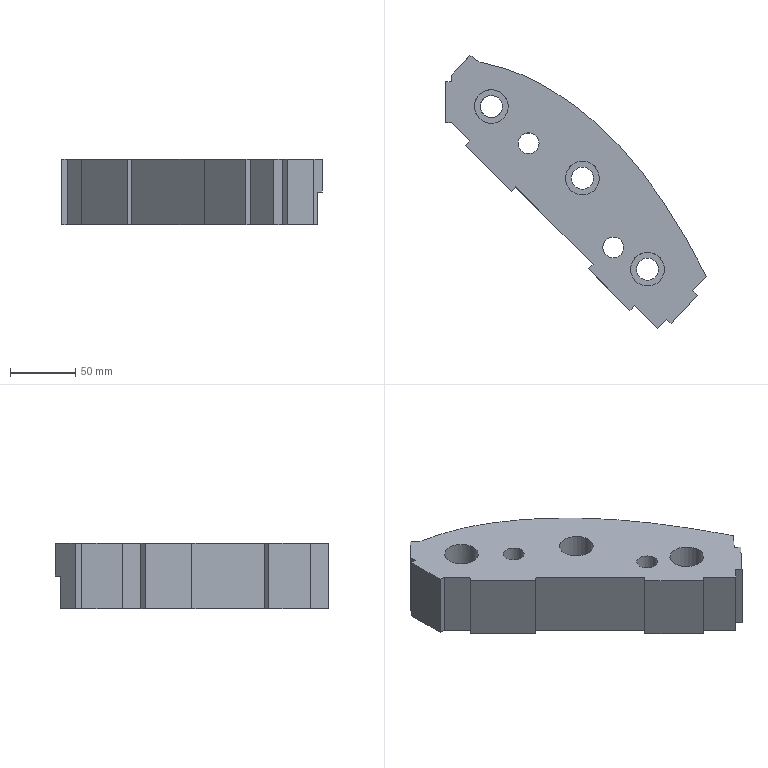Part | NX | features solid 2 | 1 solid | 37 faces | box 200.345 x 210.054 x 50 mm | volume 771106 mm3 | plane 25 | cylinder 8 | spline 4 | commonest cylinder face diameters 17 x3 26 x3 16 x2
STEP:
#1=CARTESIAN_POINT('',(339.431,588.896,-50.));
#2=VERTEX_POINT('',#1);
#3=CARTESIAN_POINT('',(339.431,583.896,-50.));
#4=VERTEX_POINT('',#3);
#5=CARTESIAN_POINT('',(339.431,588.896,-50.));
#6=DIRECTION('',(0.,-1.,0.));
#7=VECTOR('',#6,1000.);
#8=LINE('',#5,#7);
#9=EDGE_CURVE('',#2,#4,#8,.T.);
#10=ORIENTED_EDGE('',*,*,#9,.T.);
#11=CARTESIAN_POINT('',(339.431,583.896,0.));
#12=VERTEX_POINT('',#11);
#13=CARTESIAN_POINT('',(339.431,583.896,-50.));
#14=DIRECTION('',(0.,0.,1.));
#15=VECTOR('',#14,1000.);
#16=LINE('',#13,#15);
#17=EDGE_CURVE('',#4,#12,#16,.T.);
#18=ORIENTED_EDGE('',*,*,#17,.T.);
#19=CARTESIAN_POINT('',(339.431,588.896,0.));
#20=VERTEX_POINT('',#19);
#21=CARTESIAN_POINT('',(339.431,588.896,0.));
#22=DIRECTION('',(0.,-1.,0.));
#23=VECTOR('',#22,1000.);
#24=LINE('',#21,#23);
#25=EDGE_CURVE('',#20,#12,#24,.T.);
#26=ORIENTED_EDGE('',*,*,#25,.F.);
#27=CARTESIAN_POINT('',(339.431,588.896,-50.));
#28=DIRECTION('',(0.,0.,1.));
#29=VECTOR('',#28,1000.);
#30=LINE('',#27,#29);
#31=EDGE_CURVE('',#2,#20,#30,.T.);
#32=ORIENTED_EDGE('',*,*,#31,.F.);
#33=EDGE_LOOP('',(#10,#18,#26,#32));
#34=FACE_BOUND('',#33,.T.);
#35=CARTESIAN_POINT('',(339.431,588.896,-50.));
#36=DIRECTION('',(-1.,0.,0.));
#37=DIRECTION('',(0.,-1.,0.));
#38=AXIS2_PLACEMENT_3D('',#35,#36,#37);
#39=PLANE('',#38);
#40=ADVANCED_FACE('',(#34),#39,.T.);
#41=CARTESIAN_POINT('',(524.901,423.149,0.));
#42=VERTEX_POINT('',#41);
#43=CARTESIAN_POINT('',(535.345,434.348,0.));
#44=VERTEX_POINT('',#43);
#45=CARTESIAN_POINT('',(497.822,394.11,0.));
#46=DIRECTION('',(0.682,0.7314,0.));
#47=VECTOR('',#46,1000.);
#48=LINE('',#45,#47);
#49=EDGE_CURVE('',#42,#44,#48,.T.);
#50=ORIENTED_EDGE('',*,*,#49,.F.);
#51=CARTESIAN_POINT('',(524.901,423.149,-50.));
#52=VERTEX_POINT('',#51);
#53=CARTESIAN_POINT('',(524.901,423.149,-42.5));
#54=DIRECTION('',(0.,0.,1.));
#55=VECTOR('',#54,1000.);
#56=LINE('',#53,#55);
#57=EDGE_CURVE('',#52,#42,#56,.T.);
#58=ORIENTED_EDGE('',*,*,#57,.F.);
#59=CARTESIAN_POINT('',(531.721,430.462,-50.));
#60=VERTEX_POINT('',#59);
#61=CARTESIAN_POINT('',(497.822,394.11,-50.));
#62=DIRECTION('',(0.682,0.7314,0.));
#63=VECTOR('',#62,1000.);
#64=LINE('',#61,#63);
#65=EDGE_CURVE('',#52,#60,#64,.T.);
#66=ORIENTED_EDGE('',*,*,#65,.T.);
#67=CARTESIAN_POINT('',(531.721,430.462,-25.));
#68=VERTEX_POINT('',#67);
#69=CARTESIAN_POINT('',(531.721,430.462,-42.5));
#70=DIRECTION('',(0.,0.,-1.));
#71=VECTOR('',#70,1000.);
#72=LINE('',#69,#71);
#73=EDGE_CURVE('',#60,#68,#72,.F.);
#74=ORIENTED_EDGE('',*,*,#73,.T.);
#75=CARTESIAN_POINT('',(535.345,434.348,-25.));
#76=VERTEX_POINT('',#75);
#77=CARTESIAN_POINT('',(497.822,394.11,-25.));
#78=DIRECTION('',(-0.682,-0.7314,0.));
#79=VECTOR('',#78,1000.);
#80=LINE('',#77,#79);
#81=EDGE_CURVE('',#76,#68,#80,.T.);
#82=ORIENTED_EDGE('',*,*,#81,.F.);
#83=CARTESIAN_POINT('',(535.345,434.348,-50.));
#84=DIRECTION('',(0.,0.,1.));
#85=VECTOR('',#84,1000.);
#86=LINE('',#83,#85);
#87=EDGE_CURVE('',#76,#44,#86,.T.);
#88=ORIENTED_EDGE('',*,*,#87,.T.);
#89=EDGE_LOOP('',(#50,#58,#66,#74,#82,#88));
#90=FACE_BOUND('',#89,.T.);
#91=CARTESIAN_POINT('',(497.822,394.11,-50.));
#92=DIRECTION('',(0.7314,-0.682,0.));
#93=DIRECTION('',(0.682,0.7314,0.));
#94=AXIS2_PLACEMENT_3D('',#91,#92,#93);
#95=PLANE('',#94);
#96=ADVANCED_FACE('',(#90),#95,.T.);
#97=CARTESIAN_POINT('',(471.782,456.506,-50.));
#98=VERTEX_POINT('',#97);
#99=CARTESIAN_POINT('',(463.782,456.506,-50.));
#100=DIRECTION('',(0.,0.,1.));
#101=DIRECTION('',(1.,0.,0.));
#102=AXIS2_PLACEMENT_3D('',#99,#100,#101);
#103=CIRCLE('',#102,8.);
#104=EDGE_CURVE('',#98,#98,#103,.T.);
#105=ORIENTED_EDGE('',*,*,#104,.T.);
#106=EDGE_LOOP('',(#105));
#107=FACE_BOUND('',#106,.T.);
#108=CARTESIAN_POINT('',(406.782,536.506,-50.));
#109=VERTEX_POINT('',#108);
#110=CARTESIAN_POINT('',(398.782,536.506,-50.));
#111=DIRECTION('',(0.,0.,1.));
#112=DIRECTION('',(1.,0.,0.));
#113=AXIS2_PLACEMENT_3D('',#110,#111,#112);
#114=CIRCLE('',#113,8.);
#115=EDGE_CURVE('',#109,#109,#114,.T.);
#116=ORIENTED_EDGE('',*,*,#115,.T.);
#117=EDGE_LOOP('',(#116));
#118=FACE_BOUND('',#117,.T.);
#119=CARTESIAN_POINT('',(498.622,439.794,-50.));
#120=VERTEX_POINT('',#119);
#121=CARTESIAN_POINT('',(490.122,439.794,-50.));
#122=DIRECTION('',(0.,0.,1.));
#123=DIRECTION('',(1.,0.,0.));
#124=AXIS2_PLACEMENT_3D('',#121,#122,#123);
#125=CIRCLE('',#124,8.5);
#126=EDGE_CURVE('',#120,#120,#125,.T.);
#127=ORIENTED_EDGE('',*,*,#126,.T.);
#128=EDGE_LOOP('',(#127));
#129=FACE_BOUND('',#128,.T.);
#130=CARTESIAN_POINT('',(414.032,572.939,-50.));
#131=VERTEX_POINT('',#130);
#132=CARTESIAN_POINT('',(414.032,572.939,-50.));
#133=CARTESIAN_POINT('',(417.217,571.026,-50.));
#134=CARTESIAN_POINT('',(423.539,566.983,-50.));
#135=CARTESIAN_POINT('',(432.884,560.264,-50.));
#136=CARTESIAN_POINT('',(440.545,554.13,-50.));
#137=CARTESIAN_POINT('',(445.865,549.533,-50.));
#138=CARTESIAN_POINT('',(448.857,546.853,-50.));
#139=CARTESIAN_POINT('',(451.177,544.723,-50.));
#140=CARTESIAN_POINT('',(453.165,542.856,-50.));
#141=CARTESIAN_POINT('',(455.911,540.224,-50.));
#142=CARTESIAN_POINT('',(460.621,535.563,-50.));
#143=CARTESIAN_POINT('',(467.258,528.576,-50.));
#144=CARTESIAN_POINT('',(473.713,521.213,-50.));
#145=CARTESIAN_POINT('',(478.166,515.824,-50.));
#146=CARTESIAN_POINT('',(480.658,512.722,-50.));
#147=CARTESIAN_POINT('',(482.595,510.261,-50.));
#148=CARTESIAN_POINT('',(484.212,508.169,-50.));
#149=CARTESIAN_POINT('',(486.473,505.196,-50.));
#150=CARTESIAN_POINT('',(490.365,499.944,-50.));
#151=CARTESIAN_POINT('',(494.805,493.652,-50.));
#152=CARTESIAN_POINT('',(499.205,487.109,-50.));
#153=CARTESIAN_POINT('',(502.491,482.067,-50.));
#154=CARTESIAN_POINT('',(505.213,477.765,-50.));
#155=CARTESIAN_POINT('',(507.12,474.681,-50.));
#156=CARTESIAN_POINT('',(508.194,472.926,-50.));
#157=CARTESIAN_POINT('',(509.037,471.536,-50.));
#158=CARTESIAN_POINT('',(509.729,470.388,-50.));
#159=CARTESIAN_POINT('',(510.707,468.757,-50.));
#160=CARTESIAN_POINT('',(512.396,465.911,-50.));
#161=CARTESIAN_POINT('',(514.835,461.725,-50.));
#162=CARTESIAN_POINT('',(517.278,457.431,-50.));
#163=CARTESIAN_POINT('',(519.009,454.334,-50.));
#164=CARTESIAN_POINT('',(519.981,452.582,-50.));
#165=CARTESIAN_POINT('',(520.767,451.155,-50.));
#166=CARTESIAN_POINT('',(521.338,450.114,-50.));
#167=CARTESIAN_POINT('',(522.19,448.552,-50.));
#168=CARTESIAN_POINT('',(523.25,446.593,-50.));
#169=CARTESIAN_POINT('',(524.572,444.13,-50.));
#170=CARTESIAN_POINT('',(526.378,440.732,-50.));
#171=CARTESIAN_POINT('',(528.729,436.256,-50.));
#172=CARTESIAN_POINT('',(530.708,432.434,-50.));
#173=CARTESIAN_POINT('',(531.721,430.462,-50.));
#174=B_SPLINE_CURVE_WITH_KNOTS('',3,(#132,#133,#134,#135,#136,#137,#138,#139,#140,#141,#142,#143,#144,#145,#146,#147,#148,#149,#150,#151,#152,#153,#154,#155,#156,#157,#158,#159,#160,#161,#162,#163,#164,#165,#166,#167,#168,#169,#170,#171,#172,#173),.UNSPECIFIED.,.F.,.F.,(4,1,1,1,1,1,1,1,1,1,1,1,1,1,1,1,1,1,1,1,1,1,1,1,1,1,1,1,1,1,1,1,1,1,1,1,1,1,1,4),(0.,0.0625,0.125,0.1875,0.2188,0.2344,0.25,0.2656,0.2812,0.3125,0.375,0.4375,0.4688,0.4844,0.5,0.5156,0.5312,0.5625,0.625,0.6562,0.6875,0.7188,0.7344,0.7422,0.75,0.7578,0.7656,0.7812,0.8125,0.8438,0.8594,0.8672,0.875,0.8828,0.8906,0.9062,0.9219,0.9375,0.9688,1.),.UNSPECIFIED.);
#175=EDGE_CURVE('',#60,#131,#174,.F.);
#176=ORIENTED_EDGE('',*,*,#175,.F.);
#177=ORIENTED_EDGE('',*,*,#65,.F.);
#178=CARTESIAN_POINT('',(528.558,419.739,-50.));
#179=VERTEX_POINT('',#178);
#180=CARTESIAN_POINT('',(528.558,419.739,-50.));
#181=DIRECTION('',(-0.7314,0.682,0.));
#182=VECTOR('',#181,1000.);
#183=LINE('',#180,#182);
#184=EDGE_CURVE('',#179,#52,#183,.T.);
#185=ORIENTED_EDGE('',*,*,#184,.F.);
#186=CARTESIAN_POINT('',(508.299,398.013,-50.));
#187=VERTEX_POINT('',#186);
#188=CARTESIAN_POINT('',(501.479,390.7,-50.));
#189=DIRECTION('',(0.682,0.7314,0.));
#190=VECTOR('',#189,1000.);
#191=LINE('',#188,#190);
#192=EDGE_CURVE('',#187,#179,#191,.T.);
#193=ORIENTED_EDGE('',*,*,#192,.F.);
#194=CARTESIAN_POINT('',(504.642,401.423,-50.));
#195=VERTEX_POINT('',#194);
#196=CARTESIAN_POINT('',(508.299,398.013,-50.));
#197=DIRECTION('',(-0.7314,0.682,0.));
#198=VECTOR('',#197,1000.);
#199=LINE('',#196,#198);
#200=EDGE_CURVE('',#187,#195,#199,.T.);
#201=ORIENTED_EDGE('',*,*,#200,.T.);
#202=CARTESIAN_POINT('',(497.822,394.11,-50.));
#203=VERTEX_POINT('',#202);
#204=CARTESIAN_POINT('',(497.822,394.11,-50.));
#205=DIRECTION('',(0.682,0.7314,0.));
#206=VECTOR('',#205,1000.);
#207=LINE('',#204,#206);
#208=EDGE_CURVE('',#203,#195,#207,.T.);
#209=ORIENTED_EDGE('',*,*,#208,.F.);
#210=CARTESIAN_POINT('',(480.145,411.787,-50.));
#211=VERTEX_POINT('',#210);
#212=CARTESIAN_POINT('',(339.431,552.501,-50.));
#213=DIRECTION('',(0.7071,-0.7071,0.));
#214=VECTOR('',#213,1000.);
#215=LINE('',#212,#214);
#216=EDGE_CURVE('',#211,#203,#215,.T.);
#217=ORIENTED_EDGE('',*,*,#216,.F.);
#218=CARTESIAN_POINT('',(476.609,408.252,-50.));
#219=VERTEX_POINT('',#218);
#220=CARTESIAN_POINT('',(480.145,411.787,-50.));
#221=DIRECTION('',(-0.7071,-0.7071,0.));
#222=VECTOR('',#221,1000.);
#223=LINE('',#220,#222);
#224=EDGE_CURVE('',#211,#219,#223,.T.);
#225=ORIENTED_EDGE('',*,*,#224,.T.);
#226=CARTESIAN_POINT('',(444.789,440.071,-50.));
#227=VERTEX_POINT('',#226);
#228=CARTESIAN_POINT('',(335.895,548.965,-50.));
#229=DIRECTION('',(0.7071,-0.7071,0.));
#230=VECTOR('',#229,1000.);
#231=LINE('',#228,#230);
#232=EDGE_CURVE('',#227,#219,#231,.T.);
#233=ORIENTED_EDGE('',*,*,#232,.F.);
#234=CARTESIAN_POINT('',(448.325,443.607,-50.));
#235=VERTEX_POINT('',#234);
#236=CARTESIAN_POINT('',(448.325,443.607,-50.));
#237=DIRECTION('',(-0.7071,-0.7071,0.));
#238=VECTOR('',#237,1000.);
#239=LINE('',#236,#238);
#240=EDGE_CURVE('',#235,#227,#239,.T.);
#241=ORIENTED_EDGE('',*,*,#240,.F.);
#242=CARTESIAN_POINT('',(388.928,503.004,-50.));
#243=VERTEX_POINT('',#242);
#244=CARTESIAN_POINT('',(339.431,552.501,-50.));
#245=DIRECTION('',(0.7071,-0.7071,0.));
#246=VECTOR('',#245,1000.);
#247=LINE('',#244,#246);
#248=EDGE_CURVE('',#243,#235,#247,.T.);
#249=ORIENTED_EDGE('',*,*,#248,.F.);
#250=CARTESIAN_POINT('',(385.393,499.468,-50.));
#251=VERTEX_POINT('',#250);
#252=CARTESIAN_POINT('',(388.928,503.004,-50.));
#253=DIRECTION('',(-0.7071,-0.7071,0.));
#254=VECTOR('',#253,1000.);
#255=LINE('',#252,#254);
#256=EDGE_CURVE('',#243,#251,#255,.T.);
#257=ORIENTED_EDGE('',*,*,#256,.T.);
#258=CARTESIAN_POINT('',(350.037,534.823,-50.));
#259=VERTEX_POINT('',#258);
#260=CARTESIAN_POINT('',(227.001,657.86,-50.));
#261=DIRECTION('',(0.7071,-0.7071,0.));
#262=VECTOR('',#261,1000.);
#263=LINE('',#260,#262);
#264=EDGE_CURVE('',#259,#251,#263,.T.);
#265=ORIENTED_EDGE('',*,*,#264,.F.);
#266=CARTESIAN_POINT('',(353.573,538.359,-50.));
#267=VERTEX_POINT('',#266);
#268=CARTESIAN_POINT('',(353.573,538.359,-50.));
#269=DIRECTION('',(-0.7071,-0.7071,0.));
#270=VECTOR('',#269,1000.);
#271=LINE('',#268,#270);
#272=EDGE_CURVE('',#267,#259,#271,.T.);
#273=ORIENTED_EDGE('',*,*,#272,.F.);
#274=CARTESIAN_POINT('',(339.431,552.501,-50.));
#275=VERTEX_POINT('',#274);
#276=CARTESIAN_POINT('',(339.431,552.501,-50.));
#277=DIRECTION('',(0.7071,-0.7071,0.));
#278=VECTOR('',#277,1000.);
#279=LINE('',#276,#278);
#280=EDGE_CURVE('',#275,#267,#279,.T.);
#281=ORIENTED_EDGE('',*,*,#280,.F.);
#282=CARTESIAN_POINT('',(335.,552.501,-50.));
#283=VERTEX_POINT('',#282);
#284=CARTESIAN_POINT('',(334.431,552.501,-50.));
#285=DIRECTION('',(1.,0.,0.));
#286=VECTOR('',#285,1000.);
#287=LINE('',#284,#286);
#288=EDGE_CURVE('',#283,#275,#287,.T.);
#289=ORIENTED_EDGE('',*,*,#288,.F.);
#290=CARTESIAN_POINT('',(335.,583.896,-50.));
#291=VERTEX_POINT('',#290);
#292=CARTESIAN_POINT('',(335.,588.896,-50.));
#293=DIRECTION('',(0.,-1.,0.));
#294=VECTOR('',#293,1000.);
#295=LINE('',#292,#294);
#296=EDGE_CURVE('',#291,#283,#295,.T.);
#297=ORIENTED_EDGE('',*,*,#296,.F.);
#298=CARTESIAN_POINT('',(334.431,583.896,-50.));
#299=DIRECTION('',(1.,0.,0.));
#300=VECTOR('',#299,1000.);
#301=LINE('',#298,#300);
#302=EDGE_CURVE('',#291,#4,#301,.T.);
#303=ORIENTED_EDGE('',*,*,#302,.T.);
#304=ORIENTED_EDGE('',*,*,#9,.F.);
#305=CARTESIAN_POINT('',(350.241,600.489,-50.));
#306=VERTEX_POINT('',#305);
#307=CARTESIAN_POINT('',(353.668,604.163,-50.));
#308=DIRECTION('',(-0.682,-0.7314,0.));
#309=VECTOR('',#308,1000.);
#310=LINE('',#307,#309);
#311=EDGE_CURVE('',#306,#2,#310,.T.);
#312=ORIENTED_EDGE('',*,*,#311,.F.);
#313=CARTESIAN_POINT('',(350.241,600.489,-50.));
#314=CARTESIAN_POINT('',(350.838,600.033,-50.));
#315=CARTESIAN_POINT('',(351.882,599.234,-50.));
#316=CARTESIAN_POINT('',(352.817,598.518,-50.));
#317=CARTESIAN_POINT('',(353.338,598.12,-50.));
#318=CARTESIAN_POINT('',(353.628,597.897,-50.));
#319=CARTESIAN_POINT('',(353.742,597.811,-50.));
#320=CARTESIAN_POINT('',(353.856,597.722,-50.));
#321=CARTESIAN_POINT('',(353.724,597.826,-50.));
#322=CARTESIAN_POINT('',(354.018,597.596,-50.));
#323=CARTESIAN_POINT('',(354.227,597.433,-50.));
#324=CARTESIAN_POINT('',(354.597,597.144,-50.));
#325=CARTESIAN_POINT('',(355.025,596.812,-50.));
#326=CARTESIAN_POINT('',(355.332,596.576,-50.));
#327=CARTESIAN_POINT('',(355.535,596.424,-50.));
#328=CARTESIAN_POINT('',(355.577,596.391,-50.));
#329=CARTESIAN_POINT('',(355.873,596.178,-50.));
#330=CARTESIAN_POINT('',(356.177,595.968,-50.));
#331=CARTESIAN_POINT('',(356.745,595.59,-50.));
#332=CARTESIAN_POINT('',(357.514,595.128,-50.));
#333=CARTESIAN_POINT('',(358.44,594.659,-50.));
#334=CARTESIAN_POINT('',(359.432,594.243,-50.));
#335=CARTESIAN_POINT('',(360.32,593.945,-50.));
#336=CARTESIAN_POINT('',(361.022,593.744,-50.));
#337=CARTESIAN_POINT('',(361.663,593.585,-50.));
#338=CARTESIAN_POINT('',(361.936,593.527,-50.));
#339=CARTESIAN_POINT('',(362.453,593.421,-50.));
#340=CARTESIAN_POINT('',(363.01,593.314,-50.));
#341=CARTESIAN_POINT('',(363.811,593.167,-50.));
#342=CARTESIAN_POINT('',(364.249,593.086,-50.));
#343=CARTESIAN_POINT('',(364.977,592.944,-50.));
#344=CARTESIAN_POINT('',(366.286,592.671,-50.));
#345=CARTESIAN_POINT('',(367.95,592.297,-50.));
#346=CARTESIAN_POINT('',(370.764,591.624,-50.));
#347=CARTESIAN_POINT('',(374.347,590.68,-50.));
#348=CARTESIAN_POINT('',(378.549,589.448,-50.));
#349=CARTESIAN_POINT('',(382.734,588.07,-50.));
#350=CARTESIAN_POINT('',(386.64,586.652,-50.));
#351=CARTESIAN_POINT('',(391.924,584.557,-50.));
#352=CARTESIAN_POINT('',(398.466,581.625,-50.));
#353=CARTESIAN_POINT('',(406.28,577.583,-50.));
#354=CARTESIAN_POINT('',(411.453,574.545,-50.));
#355=CARTESIAN_POINT('',(414.032,572.939,-50.));
#356=B_SPLINE_CURVE_WITH_KNOTS('',3,(#313,#314,#315,#316,#317,#318,#319,#320,#321,#322,#323,#324,#325,#326,#327,#328,#329,#330,#331,#332,#333,#334,#335,#336,#337,#338,#339,#340,#341,#342,#343,#344,#345,#346,#347,#348,#349,#350,#351,#352,#353,#354,#355),.UNSPECIFIED.,.F.,.F.,(4,1,1,1,1,1,1,1,1,1,1,1,1,1,1,1,1,1,1,1,1,1,1,1,1,1,1,1,1,1,1,1,1,1,1,1,1,1,1,1,4),(0.,0.01562,0.03125,0.03906,0.04688,0.05469,0.05859,0.0625,0.06445,0.06641,0.07031,0.07812,0.08594,0.08984,0.09375,0.09766,0.1016,0.1094,0.125,0.1406,0.1562,0.1719,0.1797,0.1875,0.1953,0.2031,0.2109,0.2188,0.2266,0.2344,0.25,0.2812,0.3125,0.375,0.4375,0.5,0.5625,0.625,0.75,0.875,1.),.UNSPECIFIED.);
#357=EDGE_CURVE('',#131,#306,#356,.F.);
#358=ORIENTED_EDGE('',*,*,#357,.F.);
#359=EDGE_LOOP('',(#176,#177,#185,#193,#201,#209,#217,#225,#233,#241,#249,#257,#265,#273,#281,#289,#297,#303,#304,#312,#358));
#360=FACE_BOUND('',#359,.T.);
#361=CARTESIAN_POINT('',(448.622,509.794,-50.));
#362=VERTEX_POINT('',#361);
#363=CARTESIAN_POINT('',(440.122,509.794,-50.));
#364=DIRECTION('',(0.,0.,1.));
#365=DIRECTION('',(1.,0.,0.));
#366=AXIS2_PLACEMENT_3D('',#363,#364,#365);
#367=CIRCLE('',#366,8.5);
#368=EDGE_CURVE('',#362,#362,#367,.T.);
#369=ORIENTED_EDGE('',*,*,#368,.T.);
#370=EDGE_LOOP('',(#369));
#371=FACE_BOUND('',#370,.T.);
#372=CARTESIAN_POINT('',(378.622,564.794,-50.));
#373=VERTEX_POINT('',#372);
#374=CARTESIAN_POINT('',(370.122,564.794,-50.));
#375=DIRECTION('',(0.,0.,1.));
#376=DIRECTION('',(1.,0.,0.));
#377=AXIS2_PLACEMENT_3D('',#374,#375,#376);
#378=CIRCLE('',#377,8.5);
#379=EDGE_CURVE('',#373,#373,#378,.T.);
#380=ORIENTED_EDGE('',*,*,#379,.T.);
#381=EDGE_LOOP('',(#380));
#382=FACE_BOUND('',#381,.T.);
#383=CARTESIAN_POINT('',(327.241,1363.389,-50.));
#384=DIRECTION('',(0.,0.,1.));
#385=DIRECTION('',(1.,0.,0.));
#386=AXIS2_PLACEMENT_3D('',#383,#384,#385);
#387=PLANE('',#386);
#388=ADVANCED_FACE('',(#107,#118,#129,#360,#371,#382),#387,.F.);
#389=CARTESIAN_POINT('',(471.782,456.506,0.));
#390=VERTEX_POINT('',#389);
#391=CARTESIAN_POINT('',(463.782,456.506,0.));
#392=DIRECTION('',(0.,0.,1.));
#393=DIRECTION('',(1.,0.,0.));
#394=AXIS2_PLACEMENT_3D('',#391,#392,#393);
#395=CIRCLE('',#394,8.);
#396=EDGE_CURVE('',#390,#390,#395,.T.);
#397=ORIENTED_EDGE('',*,*,#396,.F.);
#398=EDGE_LOOP('',(#397));
#399=FACE_BOUND('',#398,.T.);
#400=CARTESIAN_POINT('',(406.782,536.506,0.));
#401=VERTEX_POINT('',#400);
#402=CARTESIAN_POINT('',(398.782,536.506,0.));
#403=DIRECTION('',(0.,0.,1.));
#404=DIRECTION('',(1.,0.,0.));
#405=AXIS2_PLACEMENT_3D('',#402,#403,#404);
#406=CIRCLE('',#405,8.);
#407=EDGE_CURVE('',#401,#401,#406,.T.);
#408=ORIENTED_EDGE('',*,*,#407,.F.);
#409=EDGE_LOOP('',(#408));
#410=FACE_BOUND('',#409,.T.);
#411=CARTESIAN_POINT('',(503.122,439.794,0.));
#412=VERTEX_POINT('',#411);
#413=CARTESIAN_POINT('',(490.122,439.794,0.));
#414=DIRECTION('',(0.,0.,1.));
#415=DIRECTION('',(1.,0.,0.));
#416=AXIS2_PLACEMENT_3D('',#413,#414,#415);
#417=CIRCLE('',#416,13.);
#418=EDGE_CURVE('',#412,#412,#417,.T.);
#419=ORIENTED_EDGE('',*,*,#418,.F.);
#420=EDGE_LOOP('',(#419));
#421=FACE_BOUND('',#420,.T.);
#422=CARTESIAN_POINT('',(497.822,394.11,0.));
#423=VERTEX_POINT('',#422);
#424=CARTESIAN_POINT('',(504.642,401.423,0.));
#425=VERTEX_POINT('',#424);
#426=CARTESIAN_POINT('',(497.822,394.11,0.));
#427=DIRECTION('',(0.682,0.7314,0.));
#428=VECTOR('',#427,1000.);
#429=LINE('',#426,#428);
#430=EDGE_CURVE('',#423,#425,#429,.T.);
#431=ORIENTED_EDGE('',*,*,#430,.T.);
#432=CARTESIAN_POINT('',(508.299,398.013,0.));
#433=VERTEX_POINT('',#432);
#434=CARTESIAN_POINT('',(508.299,398.013,0.));
#435=DIRECTION('',(-0.7314,0.682,0.));
#436=VECTOR('',#435,1000.);
#437=LINE('',#434,#436);
#438=EDGE_CURVE('',#433,#425,#437,.T.);
#439=ORIENTED_EDGE('',*,*,#438,.F.);
#440=CARTESIAN_POINT('',(528.558,419.739,0.));
#441=VERTEX_POINT('',#440);
#442=CARTESIAN_POINT('',(501.479,390.7,0.));
#443=DIRECTION('',(0.682,0.7314,0.));
#444=VECTOR('',#443,1000.);
#445=LINE('',#442,#444);
#446=EDGE_CURVE('',#433,#441,#445,.T.);
#447=ORIENTED_EDGE('',*,*,#446,.T.);
#448=CARTESIAN_POINT('',(528.558,419.739,0.));
#449=DIRECTION('',(-0.7314,0.682,0.));
#450=VECTOR('',#449,1000.);
#451=LINE('',#448,#450);
#452=EDGE_CURVE('',#441,#42,#451,.T.);
#453=ORIENTED_EDGE('',*,*,#452,.T.);
#454=ORIENTED_EDGE('',*,*,#49,.T.);
#455=CARTESIAN_POINT('',(416.641,577.204,0.));
#456=VERTEX_POINT('',#455);
#457=CARTESIAN_POINT('',(416.641,577.204,0.));
#458=CARTESIAN_POINT('',(430.085,569.129,0.));
#459=CARTESIAN_POINT('',(455.033,549.851,0.));
#460=CARTESIAN_POINT('',(486.731,514.887,0.));
#461=CARTESIAN_POINT('',(513.144,475.849,0.));
#462=CARTESIAN_POINT('',(528.174,448.296,0.));
#463=CARTESIAN_POINT('',(535.345,434.348,0.));
#464=B_SPLINE_CURVE_WITH_KNOTS('',3,(#457,#458,#459,#460,#461,#462,#463),.UNSPECIFIED.,.F.,.F.,(4,1,1,1,4),(0.2686,0.4514,0.6343,0.8171,1.),.QUASI_UNIFORM_KNOTS.);
#465=EDGE_CURVE('',#456,#44,#464,.T.);
#466=ORIENTED_EDGE('',*,*,#465,.F.);
#467=CARTESIAN_POINT('',(353.668,604.163,0.));
#468=VERTEX_POINT('',#467);
#469=CARTESIAN_POINT('',(353.668,604.163,0.));
#470=CARTESIAN_POINT('',(354.811,603.289,0.));
#471=CARTESIAN_POINT('',(356.54,601.995,0.));
#472=CARTESIAN_POINT('',(358.783,600.186,0.));
#473=CARTESIAN_POINT('',(360.642,599.063,0.));
#474=CARTESIAN_POINT('',(362.717,598.427,0.));
#475=CARTESIAN_POINT('',(365.559,597.955,0.));
#476=CARTESIAN_POINT('',(370.48,596.864,0.));
#477=CARTESIAN_POINT('',(377.452,595.064,0.));
#478=CARTESIAN_POINT('',(388.416,591.518,0.));
#479=CARTESIAN_POINT('',(401.68,585.876,0.));
#480=CARTESIAN_POINT('',(411.753,580.249,0.));
#481=CARTESIAN_POINT('',(416.641,577.204,0.));
#482=B_SPLINE_CURVE_WITH_KNOTS('',3,(#469,#470,#471,#472,#473,#474,#475,#476,#477,#478,#479,#480,#481),.UNSPECIFIED.,.F.,.F.,(4,1,1,1,1,1,1,1,1,1,4),(0.,0.01679,0.02518,0.03357,0.04197,0.05036,0.06715,0.1007,0.1343,0.2014,0.2686),.UNSPECIFIED.);
#483=EDGE_CURVE('',#468,#456,#482,.T.);
#484=ORIENTED_EDGE('',*,*,#483,.F.);
#485=CARTESIAN_POINT('',(353.668,604.163,0.));
#486=DIRECTION('',(-0.682,-0.7314,0.));
#487=VECTOR('',#486,1000.);
#488=LINE('',#485,#487);
#489=EDGE_CURVE('',#468,#20,#488,.T.);
#490=ORIENTED_EDGE('',*,*,#489,.T.);
#491=ORIENTED_EDGE('',*,*,#25,.T.);
#492=CARTESIAN_POINT('',(335.,583.896,0.));
#493=VERTEX_POINT('',#492);
#494=CARTESIAN_POINT('',(334.431,583.896,0.));
#495=DIRECTION('',(1.,0.,0.));
#496=VECTOR('',#495,1000.);
#497=LINE('',#494,#496);
#498=EDGE_CURVE('',#493,#12,#497,.T.);
#499=ORIENTED_EDGE('',*,*,#498,.F.);
#500=CARTESIAN_POINT('',(335.,552.501,0.));
#501=VERTEX_POINT('',#500);
#502=CARTESIAN_POINT('',(335.,588.896,0.));
#503=DIRECTION('',(0.,-1.,0.));
#504=VECTOR('',#503,1000.);
#505=LINE('',#502,#504);
#506=EDGE_CURVE('',#493,#501,#505,.T.);
#507=ORIENTED_EDGE('',*,*,#506,.T.);
#508=CARTESIAN_POINT('',(339.431,552.501,0.));
#509=VERTEX_POINT('',#508);
#510=CARTESIAN_POINT('',(334.431,552.501,0.));
#511=DIRECTION('',(1.,0.,0.));
#512=VECTOR('',#511,1000.);
#513=LINE('',#510,#512);
#514=EDGE_CURVE('',#501,#509,#513,.T.);
#515=ORIENTED_EDGE('',*,*,#514,.T.);
#516=CARTESIAN_POINT('',(353.573,538.359,0.));
#517=VERTEX_POINT('',#516);
#518=CARTESIAN_POINT('',(339.431,552.501,0.));
#519=DIRECTION('',(0.7071,-0.7071,0.));
#520=VECTOR('',#519,1000.);
#521=LINE('',#518,#520);
#522=EDGE_CURVE('',#509,#517,#521,.T.);
#523=ORIENTED_EDGE('',*,*,#522,.T.);
#524=CARTESIAN_POINT('',(350.037,534.823,0.));
#525=VERTEX_POINT('',#524);
#526=CARTESIAN_POINT('',(353.573,538.359,0.));
#527=DIRECTION('',(-0.7071,-0.7071,0.));
#528=VECTOR('',#527,1000.);
#529=LINE('',#526,#528);
#530=EDGE_CURVE('',#517,#525,#529,.T.);
#531=ORIENTED_EDGE('',*,*,#530,.T.);
#532=CARTESIAN_POINT('',(385.393,499.468,0.));
#533=VERTEX_POINT('',#532);
#534=CARTESIAN_POINT('',(227.001,657.86,0.));
#535=DIRECTION('',(0.7071,-0.7071,0.));
#536=VECTOR('',#535,1000.);
#537=LINE('',#534,#536);
#538=EDGE_CURVE('',#525,#533,#537,.T.);
#539=ORIENTED_EDGE('',*,*,#538,.T.);
#540=CARTESIAN_POINT('',(388.928,503.004,0.));
#541=VERTEX_POINT('',#540);
#542=CARTESIAN_POINT('',(388.928,503.004,0.));
#543=DIRECTION('',(-0.7071,-0.7071,0.));
#544=VECTOR('',#543,1000.);
#545=LINE('',#542,#544);
#546=EDGE_CURVE('',#541,#533,#545,.T.);
#547=ORIENTED_EDGE('',*,*,#546,.F.);
#548=CARTESIAN_POINT('',(448.325,443.607,0.));
#549=VERTEX_POINT('',#548);
#550=CARTESIAN_POINT('',(339.431,552.501,0.));
#551=DIRECTION('',(0.7071,-0.7071,0.));
#552=VECTOR('',#551,1000.);
#553=LINE('',#550,#552);
#554=EDGE_CURVE('',#541,#549,#553,.T.);
#555=ORIENTED_EDGE('',*,*,#554,.T.);
#556=CARTESIAN_POINT('',(444.789,440.071,0.));
#557=VERTEX_POINT('',#556);
#558=CARTESIAN_POINT('',(448.325,443.607,0.));
#559=DIRECTION('',(-0.7071,-0.7071,0.));
#560=VECTOR('',#559,1000.);
#561=LINE('',#558,#560);
#562=EDGE_CURVE('',#549,#557,#561,.T.);
#563=ORIENTED_EDGE('',*,*,#562,.T.);
#564=CARTESIAN_POINT('',(476.609,408.252,0.));
#565=VERTEX_POINT('',#564);
#566=CARTESIAN_POINT('',(335.895,548.965,0.));
#567=DIRECTION('',(0.7071,-0.7071,0.));
#568=VECTOR('',#567,1000.);
#569=LINE('',#566,#568);
#570=EDGE_CURVE('',#557,#565,#569,.T.);
#571=ORIENTED_EDGE('',*,*,#570,.T.);
#572=CARTESIAN_POINT('',(480.145,411.787,0.));
#573=VERTEX_POINT('',#572);
#574=CARTESIAN_POINT('',(480.145,411.787,0.));
#575=DIRECTION('',(-0.7071,-0.7071,0.));
#576=VECTOR('',#575,1000.);
#577=LINE('',#574,#576);
#578=EDGE_CURVE('',#573,#565,#577,.T.);
#579=ORIENTED_EDGE('',*,*,#578,.F.);
#580=CARTESIAN_POINT('',(339.431,552.501,0.));
#581=DIRECTION('',(0.7071,-0.7071,0.));
#582=VECTOR('',#581,1000.);
#583=LINE('',#580,#582);
#584=EDGE_CURVE('',#573,#423,#583,.T.);
#585=ORIENTED_EDGE('',*,*,#584,.T.);
#586=EDGE_LOOP('',(#431,#439,#447,#453,#454,#466,#484,#490,#491,#499,#507,#515,#523,#531,#539,#547,#555,#563,#571,#579,#585));
#587=FACE_BOUND('',#586,.T.);
#588=CARTESIAN_POINT('',(453.122,509.794,0.));
#589=VERTEX_POINT('',#588);
#590=CARTESIAN_POINT('',(440.122,509.794,0.));
#591=DIRECTION('',(0.,0.,1.));
#592=DIRECTION('',(1.,0.,0.));
#593=AXIS2_PLACEMENT_3D('',#590,#591,#592);
#594=CIRCLE('',#593,13.);
#595=EDGE_CURVE('',#589,#589,#594,.T.);
#596=ORIENTED_EDGE('',*,*,#595,.F.);
#597=EDGE_LOOP('',(#596));
#598=FACE_BOUND('',#597,.T.);
#599=CARTESIAN_POINT('',(383.122,564.794,0.));
#600=VERTEX_POINT('',#599);
#601=CARTESIAN_POINT('',(370.122,564.794,0.));
#602=DIRECTION('',(0.,0.,1.));
#603=DIRECTION('',(1.,0.,0.));
#604=AXIS2_PLACEMENT_3D('',#601,#602,#603);
#605=CIRCLE('',#604,13.);
#606=EDGE_CURVE('',#600,#600,#605,.T.);
#607=ORIENTED_EDGE('',*,*,#606,.F.);
#608=EDGE_LOOP('',(#607));
#609=FACE_BOUND('',#608,.T.);
#610=CARTESIAN_POINT('',(327.241,1363.389,0.));
#611=DIRECTION('',(0.,0.,1.));
#612=DIRECTION('',(1.,0.,0.));
#613=AXIS2_PLACEMENT_3D('',#610,#611,#612);
#614=PLANE('',#613);
#615=ADVANCED_FACE('',(#399,#410,#421,#587,#598,#609),#614,.T.);
#616=CARTESIAN_POINT('',(414.032,572.939,-25.));
#617=VERTEX_POINT('',#616);
#618=CARTESIAN_POINT('',(414.032,572.939,-25.));
#619=CARTESIAN_POINT('',(415.729,571.919,-25.));
#620=CARTESIAN_POINT('',(418.95,569.92,-25.));
#621=CARTESIAN_POINT('',(425.426,565.639,-25.));
#622=CARTESIAN_POINT('',(433.254,559.981,-25.));
#623=CARTESIAN_POINT('',(442.325,552.687,-25.));
#624=CARTESIAN_POINT('',(453.952,542.379,-25.));
#625=CARTESIAN_POINT('',(467.619,528.527,-25.));
#626=CARTESIAN_POINT('',(487.683,504.642,-25.));
#627=CARTESIAN_POINT('',(505.161,478.651,-25.));
#628=CARTESIAN_POINT('',(520.799,451.399,-25.));
#629=CARTESIAN_POINT('',(528.101,437.504,-25.));
#630=CARTESIAN_POINT('',(531.721,430.462,-25.));
#631=B_SPLINE_CURVE_WITH_KNOTS('',3,(#618,#619,#620,#621,#622,#623,#624,#625,#626,#627,#628,#629,#630),.UNSPECIFIED.,.F.,.F.,(4,1,1,1,1,1,1,1,1,1,4),(-0.0002141,0.03134,0.0629,0.126,0.1891,0.2522,0.3785,0.5047,0.7571,0.8833,1.01),.UNSPECIFIED.);
#632=EDGE_CURVE('',#617,#68,#631,.T.);
#633=ORIENTED_EDGE('',*,*,#632,.F.);
#634=CARTESIAN_POINT('',(350.241,600.489,-25.));
#635=VERTEX_POINT('',#634);
#636=CARTESIAN_POINT('',(350.241,600.489,-25.));
#637=CARTESIAN_POINT('',(350.817,600.049,-25.));
#638=CARTESIAN_POINT('',(352.,599.149,-25.));
#639=CARTESIAN_POINT('',(353.403,598.082,-25.));
#640=CARTESIAN_POINT('',(354.469,597.238,-25.));
#641=CARTESIAN_POINT('',(355.788,596.209,-25.));
#642=CARTESIAN_POINT('',(357.485,595.068,-25.));
#643=CARTESIAN_POINT('',(359.598,594.158,-25.));
#644=CARTESIAN_POINT('',(361.571,593.565,-25.));
#645=CARTESIAN_POINT('',(363.297,593.263,-25.));
#646=CARTESIAN_POINT('',(364.564,593.028,-25.));
#647=CARTESIAN_POINT('',(365.9,592.755,-25.));
#648=CARTESIAN_POINT('',(367.587,592.376,-25.));
#649=CARTESIAN_POINT('',(369.658,591.883,-25.));
#650=CARTESIAN_POINT('',(372.386,591.198,-25.));
#651=CARTESIAN_POINT('',(375.772,590.277,-25.));
#652=CARTESIAN_POINT('',(379.788,589.053,-25.));
#653=CARTESIAN_POINT('',(385.096,587.258,-25.));
#654=CARTESIAN_POINT('',(391.627,584.717,-25.));
#655=CARTESIAN_POINT('',(399.298,581.215,-25.));
#656=CARTESIAN_POINT('',(405.522,577.957,-25.));
#657=CARTESIAN_POINT('',(410.437,575.139,-25.));
#658=CARTESIAN_POINT('',(412.801,573.706,-25.));
#659=CARTESIAN_POINT('',(414.032,572.939,-25.));
#660=B_SPLINE_CURVE_WITH_KNOTS('',3,(#636,#637,#638,#639,#640,#641,#642,#643,#644,#645,#646,#647,#648,#649,#650,#651,#652,#653,#654,#655,#656,#657,#658,#659),.UNSPECIFIED.,.F.,.F.,(4,1,1,1,1,1,1,1,1,1,1,1,1,1,1,1,1,1,1,1,1,4),(-0.007061,0.02443,0.05592,0.07166,0.08741,0.1189,0.1346,0.1504,0.1819,0.1976,0.2134,0.2449,0.2763,0.3078,0.3708,0.4338,0.4968,0.6227,0.7487,0.8746,0.9376,1.001),.UNSPECIFIED.);
#661=EDGE_CURVE('',#635,#617,#660,.T.);
#662=ORIENTED_EDGE('',*,*,#661,.F.);
#663=CARTESIAN_POINT('',(353.668,604.163,-25.));
#664=VERTEX_POINT('',#663);
#665=CARTESIAN_POINT('',(353.668,604.163,-25.));
#666=DIRECTION('',(0.682,0.7314,0.));
#667=VECTOR('',#666,1000.);
#668=LINE('',#665,#667);
#669=EDGE_CURVE('',#635,#664,#668,.T.);
#670=ORIENTED_EDGE('',*,*,#669,.T.);
#671=CARTESIAN_POINT('',(416.641,577.204,-25.));
#672=VERTEX_POINT('',#671);
#673=CARTESIAN_POINT('',(353.668,604.163,-25.));
#674=CARTESIAN_POINT('',(354.811,603.289,-25.));
#675=CARTESIAN_POINT('',(356.54,601.995,-25.));
#676=CARTESIAN_POINT('',(358.783,600.186,-25.));
#677=CARTESIAN_POINT('',(360.642,599.063,-25.));
#678=CARTESIAN_POINT('',(362.717,598.427,-25.));
#679=CARTESIAN_POINT('',(365.559,597.955,-25.));
#680=CARTESIAN_POINT('',(370.48,596.864,-25.));
#681=CARTESIAN_POINT('',(377.452,595.064,-25.));
#682=CARTESIAN_POINT('',(388.416,591.518,-25.));
#683=CARTESIAN_POINT('',(401.68,585.876,-25.));
#684=CARTESIAN_POINT('',(411.753,580.249,-25.));
#685=CARTESIAN_POINT('',(416.641,577.204,-25.));
#686=B_SPLINE_CURVE_WITH_KNOTS('',3,(#673,#674,#675,#676,#677,#678,#679,#680,#681,#682,#683,#684,#685),.UNSPECIFIED.,.F.,.F.,(4,1,1,1,1,1,1,1,1,1,4),(0.,0.01679,0.02518,0.03357,0.04197,0.05036,0.06715,0.1007,0.1343,0.2014,0.2686),.UNSPECIFIED.);
#687=EDGE_CURVE('',#672,#664,#686,.F.);
#688=ORIENTED_EDGE('',*,*,#687,.F.);
#689=CARTESIAN_POINT('',(416.641,577.204,-25.));
#690=CARTESIAN_POINT('',(430.085,569.129,-25.));
#691=CARTESIAN_POINT('',(455.033,549.851,-25.));
#692=CARTESIAN_POINT('',(486.731,514.887,-25.));
#693=CARTESIAN_POINT('',(513.144,475.849,-25.));
#694=CARTESIAN_POINT('',(528.174,448.296,-25.));
#695=CARTESIAN_POINT('',(535.345,434.348,-25.));
#696=B_SPLINE_CURVE_WITH_KNOTS('',3,(#689,#690,#691,#692,#693,#694,#695),.UNSPECIFIED.,.F.,.F.,(4,1,1,1,4),(0.2686,0.4514,0.6343,0.8171,1.),.QUASI_UNIFORM_KNOTS.);
#697=EDGE_CURVE('',#76,#672,#696,.F.);
#698=ORIENTED_EDGE('',*,*,#697,.F.);
#699=ORIENTED_EDGE('',*,*,#81,.T.);
#700=EDGE_LOOP('',(#633,#662,#670,#688,#698,#699));
#701=FACE_BOUND('',#700,.T.);
#702=CARTESIAN_POINT('',(353.668,604.163,-25.));
#703=DIRECTION('',(0.,0.,-1.));
#704=DIRECTION('',(-1.,0.,0.));
#705=AXIS2_PLACEMENT_3D('',#702,#703,#704);
#706=PLANE('',#705);
#707=ADVANCED_FACE('',(#701),#706,.T.);
#708=ORIENTED_EDGE('',*,*,#606,.T.);
#709=EDGE_LOOP('',(#708));
#710=FACE_BOUND('',#709,.T.);
#711=CARTESIAN_POINT('',(370.122,551.794,-25.));
#712=VERTEX_POINT('',#711);
#713=CARTESIAN_POINT('',(370.122,564.794,-25.));
#714=DIRECTION('',(0.,0.,1.));
#715=DIRECTION('',(0.,-1.,0.));
#716=AXIS2_PLACEMENT_3D('',#713,#714,#715);
#717=CIRCLE('',#716,13.);
#718=EDGE_CURVE('',#712,#712,#717,.T.);
#719=ORIENTED_EDGE('',*,*,#718,.F.);
#720=EDGE_LOOP('',(#719));
#721=FACE_BOUND('',#720,.T.);
#722=CARTESIAN_POINT('',(370.122,564.794,-25.));
#723=DIRECTION('',(0.,0.,1.));
#724=DIRECTION('',(0.,-1.,0.));
#725=AXIS2_PLACEMENT_3D('',#722,#723,#724);
#726=CYLINDRICAL_SURFACE('',#725,13.);
#727=ADVANCED_FACE('',(#710,#721),#726,.F.);
#728=CARTESIAN_POINT('',(370.122,573.294,-25.));
#729=VERTEX_POINT('',#728);
#730=CARTESIAN_POINT('',(370.122,564.794,-25.));
#731=DIRECTION('',(0.,0.,-1.));
#732=DIRECTION('',(0.,1.,0.));
#733=AXIS2_PLACEMENT_3D('',#730,#731,#732);
#734=CIRCLE('',#733,8.5);
#735=EDGE_CURVE('',#729,#729,#734,.F.);
#736=ORIENTED_EDGE('',*,*,#735,.F.);
#737=EDGE_LOOP('',(#736));
#738=FACE_BOUND('',#737,.T.);
#739=ORIENTED_EDGE('',*,*,#718,.T.);
#740=EDGE_LOOP('',(#739));
#741=FACE_BOUND('',#740,.T.);
#742=CARTESIAN_POINT('',(370.122,564.794,-25.));
#743=DIRECTION('',(0.,0.,-1.));
#744=DIRECTION('',(0.,1.,0.));
#745=AXIS2_PLACEMENT_3D('',#742,#743,#744);
#746=PLANE('',#745);
#747=ADVANCED_FACE('',(#738,#741),#746,.F.);
#748=ORIENTED_EDGE('',*,*,#379,.F.);
#749=EDGE_LOOP('',(#748));
#750=FACE_BOUND('',#749,.T.);
#751=ORIENTED_EDGE('',*,*,#735,.T.);
#752=EDGE_LOOP('',(#751));
#753=FACE_BOUND('',#752,.T.);
#754=CARTESIAN_POINT('',(370.122,564.794,-75.));
#755=DIRECTION('',(0.,0.,1.));
#756=DIRECTION('',(0.,-1.,0.));
#757=AXIS2_PLACEMENT_3D('',#754,#755,#756);
#758=CYLINDRICAL_SURFACE('',#757,8.5);
#759=ADVANCED_FACE('',(#750,#753),#758,.F.);
#760=ORIENTED_EDGE('',*,*,#595,.T.);
#761=EDGE_LOOP('',(#760));
#762=FACE_BOUND('',#761,.T.);
#763=CARTESIAN_POINT('',(453.122,509.794,-25.));
#764=VERTEX_POINT('',#763);
#765=CARTESIAN_POINT('',(440.122,509.794,-25.));
#766=DIRECTION('',(0.,0.,1.));
#767=DIRECTION('',(1.,0.,0.));
#768=AXIS2_PLACEMENT_3D('',#765,#766,#767);
#769=CIRCLE('',#768,13.);
#770=EDGE_CURVE('',#764,#764,#769,.T.);
#771=ORIENTED_EDGE('',*,*,#770,.F.);
#772=EDGE_LOOP('',(#771));
#773=FACE_BOUND('',#772,.T.);
#774=CARTESIAN_POINT('',(440.122,509.794,-25.));
#775=DIRECTION('',(0.,0.,1.));
#776=DIRECTION('',(1.,0.,0.));
#777=AXIS2_PLACEMENT_3D('',#774,#775,#776);
#778=CYLINDRICAL_SURFACE('',#777,13.);
#779=ADVANCED_FACE('',(#762,#773),#778,.F.);
#780=CARTESIAN_POINT('',(431.622,509.794,-25.));
#781=VERTEX_POINT('',#780);
#782=CARTESIAN_POINT('',(440.122,509.794,-25.));
#783=DIRECTION('',(0.,0.,-1.));
#784=DIRECTION('',(-1.,0.,0.));
#785=AXIS2_PLACEMENT_3D('',#782,#783,#784);
#786=CIRCLE('',#785,8.5);
#787=EDGE_CURVE('',#781,#781,#786,.F.);
#788=ORIENTED_EDGE('',*,*,#787,.F.);
#789=EDGE_LOOP('',(#788));
#790=FACE_BOUND('',#789,.T.);
#791=ORIENTED_EDGE('',*,*,#770,.T.);
#792=EDGE_LOOP('',(#791));
#793=FACE_BOUND('',#792,.T.);
#794=CARTESIAN_POINT('',(440.122,509.794,-25.));
#795=DIRECTION('',(0.,0.,-1.));
#796=DIRECTION('',(-1.,0.,0.));
#797=AXIS2_PLACEMENT_3D('',#794,#795,#796);
#798=PLANE('',#797);
#799=ADVANCED_FACE('',(#790,#793),#798,.F.);
#800=ORIENTED_EDGE('',*,*,#368,.F.);
#801=EDGE_LOOP('',(#800));
#802=FACE_BOUND('',#801,.T.);
#803=ORIENTED_EDGE('',*,*,#787,.T.);
#804=EDGE_LOOP('',(#803));
#805=FACE_BOUND('',#804,.T.);
#806=CARTESIAN_POINT('',(440.122,509.794,-75.));
#807=DIRECTION('',(0.,0.,1.));
#808=DIRECTION('',(1.,0.,0.));
#809=AXIS2_PLACEMENT_3D('',#806,#807,#808);
#810=CYLINDRICAL_SURFACE('',#809,8.5);
#811=ADVANCED_FACE('',(#802,#805),#810,.F.);
#812=ORIENTED_EDGE('',*,*,#175,.T.);
#813=CARTESIAN_POINT('',(414.032,572.939,-42.5));
#814=DIRECTION('',(0.,0.,-1.));
#815=VECTOR('',#814,1000.);
#816=LINE('',#813,#815);
#817=EDGE_CURVE('',#617,#131,#816,.T.);
#818=ORIENTED_EDGE('',*,*,#817,.F.);
#819=ORIENTED_EDGE('',*,*,#632,.T.);
#820=ORIENTED_EDGE('',*,*,#73,.F.);
#821=EDGE_LOOP('',(#812,#818,#819,#820));
#822=FACE_BOUND('',#821,.T.);
#823=CARTESIAN_POINT('',(414.032,572.939,-25.));
#824=CARTESIAN_POINT('',(414.032,572.939,-50.));
#825=CARTESIAN_POINT('',(415.729,571.919,-25.));
#826=CARTESIAN_POINT('',(415.729,571.919,-50.));
#827=CARTESIAN_POINT('',(418.95,569.92,-25.));
#828=CARTESIAN_POINT('',(418.95,569.92,-50.));
#829=CARTESIAN_POINT('',(425.426,565.639,-25.));
#830=CARTESIAN_POINT('',(425.426,565.639,-50.));
#831=CARTESIAN_POINT('',(433.254,559.981,-25.));
#832=CARTESIAN_POINT('',(433.254,559.981,-50.));
#833=CARTESIAN_POINT('',(442.325,552.687,-25.));
#834=CARTESIAN_POINT('',(442.325,552.687,-50.));
#835=CARTESIAN_POINT('',(453.952,542.379,-25.));
#836=CARTESIAN_POINT('',(453.952,542.379,-50.));
#837=CARTESIAN_POINT('',(467.619,528.527,-25.));
#838=CARTESIAN_POINT('',(467.619,528.527,-50.));
#839=CARTESIAN_POINT('',(487.683,504.642,-25.));
#840=CARTESIAN_POINT('',(487.683,504.642,-50.));
#841=CARTESIAN_POINT('',(505.161,478.651,-25.));
#842=CARTESIAN_POINT('',(505.161,478.651,-50.));
#843=CARTESIAN_POINT('',(520.799,451.399,-25.));
#844=CARTESIAN_POINT('',(520.799,451.399,-50.));
#845=CARTESIAN_POINT('',(528.101,437.504,-25.));
#846=CARTESIAN_POINT('',(528.101,437.504,-50.));
#847=CARTESIAN_POINT('',(531.721,430.462,-25.));
#848=CARTESIAN_POINT('',(531.721,430.462,-50.));
#849=B_SPLINE_SURFACE_WITH_KNOTS('',3,1,((#823,#824),(#825,#826),(#827,#828),(#829,#830),(#831,#832),(#833,#834),(#835,#836),(#837,#838),(#839,#840),(#841,#842),(#843,#844),(#845,#846),(#847,#848)),.SURF_OF_LINEAR_EXTRUSION.,.F.,.F.,.F.,(4,1,1,1,1,1,1,1,1,1,4),(2,2),(-0.0002141,0.03134,0.0629,0.126,0.1891,0.2522,0.3785,0.5047,0.7571,0.8833,1.01),(0.,1.),.UNSPECIFIED.);
#850=ADVANCED_FACE('',(#822),#849,.T.);
#851=ORIENTED_EDGE('',*,*,#697,.T.);
#852=CARTESIAN_POINT('',(416.641,577.204,-50.));
#853=DIRECTION('',(0.,0.,1.));
#854=VECTOR('',#853,1000.);
#855=LINE('',#852,#854);
#856=EDGE_CURVE('',#672,#456,#855,.T.);
#857=ORIENTED_EDGE('',*,*,#856,.T.);
#858=ORIENTED_EDGE('',*,*,#465,.T.);
#859=ORIENTED_EDGE('',*,*,#87,.F.);
#860=EDGE_LOOP('',(#851,#857,#858,#859));
#861=FACE_BOUND('',#860,.T.);
#862=CARTESIAN_POINT('',(416.641,577.204,-25.));
#863=CARTESIAN_POINT('',(416.641,577.204,0.));
#864=CARTESIAN_POINT('',(430.085,569.129,-25.));
#865=CARTESIAN_POINT('',(430.085,569.129,0.));
#866=CARTESIAN_POINT('',(455.033,549.851,-25.));
#867=CARTESIAN_POINT('',(455.033,549.851,0.));
#868=CARTESIAN_POINT('',(486.731,514.887,-25.));
#869=CARTESIAN_POINT('',(486.731,514.887,0.));
#870=CARTESIAN_POINT('',(513.144,475.849,-25.));
#871=CARTESIAN_POINT('',(513.144,475.849,0.));
#872=CARTESIAN_POINT('',(528.174,448.296,-25.));
#873=CARTESIAN_POINT('',(528.174,448.296,0.));
#874=CARTESIAN_POINT('',(535.345,434.348,-25.));
#875=CARTESIAN_POINT('',(535.345,434.348,0.));
#876=B_SPLINE_SURFACE_WITH_KNOTS('',3,1,((#862,#863),(#864,#865),(#866,#867),(#868,#869),(#870,#871),(#872,#873),(#874,#875)),.SURF_OF_LINEAR_EXTRUSION.,.F.,.F.,.F.,(4,1,1,1,4),(2,2),(0.2686,0.4514,0.6343,0.8171,1.),(0.,1.),.UNSPECIFIED.);
#877=ADVANCED_FACE('',(#861),#876,.F.);
#878=ORIENTED_EDGE('',*,*,#418,.T.);
#879=EDGE_LOOP('',(#878));
#880=FACE_BOUND('',#879,.T.);
#881=CARTESIAN_POINT('',(503.122,439.794,-25.));
#882=VERTEX_POINT('',#881);
#883=CARTESIAN_POINT('',(490.122,439.794,-25.));
#884=DIRECTION('',(0.,0.,1.));
#885=DIRECTION('',(1.,0.,0.));
#886=AXIS2_PLACEMENT_3D('',#883,#884,#885);
#887=CIRCLE('',#886,13.);
#888=EDGE_CURVE('',#882,#882,#887,.T.);
#889=ORIENTED_EDGE('',*,*,#888,.F.);
#890=EDGE_LOOP('',(#889));
#891=FACE_BOUND('',#890,.T.);
#892=CARTESIAN_POINT('',(490.122,439.794,-25.));
#893=DIRECTION('',(0.,0.,1.));
#894=DIRECTION('',(1.,0.,0.));
#895=AXIS2_PLACEMENT_3D('',#892,#893,#894);
#896=CYLINDRICAL_SURFACE('',#895,13.);
#897=ADVANCED_FACE('',(#880,#891),#896,.F.);
#898=ORIENTED_EDGE('',*,*,#888,.T.);
#899=EDGE_LOOP('',(#898));
#900=FACE_BOUND('',#899,.T.);
#901=CARTESIAN_POINT('',(481.622,439.794,-25.));
#902=VERTEX_POINT('',#901);
#903=CARTESIAN_POINT('',(490.122,439.794,-25.));
#904=DIRECTION('',(0.,0.,-1.));
#905=DIRECTION('',(-1.,0.,0.));
#906=AXIS2_PLACEMENT_3D('',#903,#904,#905);
#907=CIRCLE('',#906,8.5);
#908=EDGE_CURVE('',#902,#902,#907,.F.);
#909=ORIENTED_EDGE('',*,*,#908,.F.);
#910=EDGE_LOOP('',(#909));
#911=FACE_BOUND('',#910,.T.);
#912=CARTESIAN_POINT('',(490.122,439.794,-25.));
#913=DIRECTION('',(0.,0.,-1.));
#914=DIRECTION('',(-1.,0.,0.));
#915=AXIS2_PLACEMENT_3D('',#912,#913,#914);
#916=PLANE('',#915);
#917=ADVANCED_FACE('',(#900,#911),#916,.F.);
#918=ORIENTED_EDGE('',*,*,#908,.T.);
#919=EDGE_LOOP('',(#918));
#920=FACE_BOUND('',#919,.T.);
#921=ORIENTED_EDGE('',*,*,#126,.F.);
#922=EDGE_LOOP('',(#921));
#923=FACE_BOUND('',#922,.T.);
#924=CARTESIAN_POINT('',(490.122,439.794,-75.));
#925=DIRECTION('',(0.,0.,1.));
#926=DIRECTION('',(1.,0.,0.));
#927=AXIS2_PLACEMENT_3D('',#924,#925,#926);
#928=CYLINDRICAL_SURFACE('',#927,8.5);
#929=ADVANCED_FACE('',(#920,#923),#928,.F.);
#930=ORIENTED_EDGE('',*,*,#264,.T.);
#931=CARTESIAN_POINT('',(385.393,499.468,-50.));
#932=DIRECTION('',(0.,0.,1.));
#933=VECTOR('',#932,1000.);
#934=LINE('',#931,#933);
#935=EDGE_CURVE('',#251,#533,#934,.T.);
#936=ORIENTED_EDGE('',*,*,#935,.T.);
#937=ORIENTED_EDGE('',*,*,#538,.F.);
#938=CARTESIAN_POINT('',(350.037,534.823,-50.));
#939=DIRECTION('',(0.,0.,1.));
#940=VECTOR('',#939,1000.);
#941=LINE('',#938,#940);
#942=EDGE_CURVE('',#259,#525,#941,.T.);
#943=ORIENTED_EDGE('',*,*,#942,.F.);
#944=EDGE_LOOP('',(#930,#936,#937,#943));
#945=FACE_BOUND('',#944,.T.);
#946=CARTESIAN_POINT('',(227.001,657.86,-50.));
#947=DIRECTION('',(-0.7071,-0.7071,0.));
#948=DIRECTION('',(0.7071,-0.7071,0.));
#949=AXIS2_PLACEMENT_3D('',#946,#947,#948);
#950=PLANE('',#949);
#951=ADVANCED_FACE('',(#945),#950,.T.);
#952=ORIENTED_EDGE('',*,*,#942,.T.);
#953=ORIENTED_EDGE('',*,*,#530,.F.);
#954=CARTESIAN_POINT('',(353.573,538.359,-50.));
#955=DIRECTION('',(0.,0.,1.));
#956=VECTOR('',#955,1000.);
#957=LINE('',#954,#956);
#958=EDGE_CURVE('',#267,#517,#957,.T.);
#959=ORIENTED_EDGE('',*,*,#958,.F.);
#960=ORIENTED_EDGE('',*,*,#272,.T.);
#961=EDGE_LOOP('',(#952,#953,#959,#960));
#962=FACE_BOUND('',#961,.T.);
#963=CARTESIAN_POINT('',(353.573,538.359,-50.));
#964=DIRECTION('',(0.7071,-0.7071,0.));
#965=DIRECTION('',(0.7071,0.7071,0.));
#966=AXIS2_PLACEMENT_3D('',#963,#964,#965);
#967=PLANE('',#966);
#968=ADVANCED_FACE('',(#962),#967,.F.);
#969=ORIENTED_EDGE('',*,*,#280,.T.);
#970=ORIENTED_EDGE('',*,*,#958,.T.);
#971=ORIENTED_EDGE('',*,*,#522,.F.);
#972=CARTESIAN_POINT('',(339.431,552.501,-50.));
#973=DIRECTION('',(0.,0.,1.));
#974=VECTOR('',#973,1000.);
#975=LINE('',#972,#974);
#976=EDGE_CURVE('',#275,#509,#975,.T.);
#977=ORIENTED_EDGE('',*,*,#976,.F.);
#978=EDGE_LOOP('',(#969,#970,#971,#977));
#979=FACE_BOUND('',#978,.T.);
#980=CARTESIAN_POINT('',(339.431,552.501,-50.));
#981=DIRECTION('',(-0.7071,-0.7071,0.));
#982=DIRECTION('',(0.7071,-0.7071,0.));
#983=AXIS2_PLACEMENT_3D('',#980,#981,#982);
#984=PLANE('',#983);
#985=ADVANCED_FACE('',(#979),#984,.T.);
#986=ORIENTED_EDGE('',*,*,#483,.T.);
#987=ORIENTED_EDGE('',*,*,#856,.F.);
#988=ORIENTED_EDGE('',*,*,#687,.T.);
#989=CARTESIAN_POINT('',(353.668,604.163,-70.));
#990=DIRECTION('',(0.,0.,1.));
#991=VECTOR('',#990,1000.);
#992=LINE('',#989,#991);
#993=EDGE_CURVE('',#664,#468,#992,.T.);
#994=ORIENTED_EDGE('',*,*,#993,.T.);
#995=EDGE_LOOP('',(#986,#987,#988,#994));
#996=FACE_BOUND('',#995,.T.);
#997=CARTESIAN_POINT('',(353.668,604.163,-25.));
#998=CARTESIAN_POINT('',(353.668,604.163,0.));
#999=CARTESIAN_POINT('',(354.811,603.289,-25.));
#1000=CARTESIAN_POINT('',(354.811,603.289,0.));
#1001=CARTESIAN_POINT('',(357.095,601.566,-25.));
#1002=CARTESIAN_POINT('',(357.095,601.566,0.));
#1003=CARTESIAN_POINT('',(360.526,598.8,-25.));
#1004=CARTESIAN_POINT('',(360.526,598.8,0.));
#1005=CARTESIAN_POINT('',(364.87,598.096,-25.));
#1006=CARTESIAN_POINT('',(364.87,598.096,0.));
#1007=CARTESIAN_POINT('',(369.07,597.18,-25.));
#1008=CARTESIAN_POINT('',(369.07,597.18,0.));
#1009=CARTESIAN_POINT('',(373.27,596.143,-25.));
#1010=CARTESIAN_POINT('',(373.27,596.143,0.));
#1011=CARTESIAN_POINT('',(378.822,594.622,-25.));
#1012=CARTESIAN_POINT('',(378.822,594.622,0.));
#1013=CARTESIAN_POINT('',(385.675,592.404,-25.));
#1014=CARTESIAN_POINT('',(385.675,592.404,0.));
#1015=CARTESIAN_POINT('',(393.722,589.261,-25.));
#1016=CARTESIAN_POINT('',(393.722,589.261,0.));
#1017=CARTESIAN_POINT('',(404.198,584.469,-25.));
#1018=CARTESIAN_POINT('',(404.198,584.469,0.));
#1019=CARTESIAN_POINT('',(411.753,580.249,-25.));
#1020=CARTESIAN_POINT('',(411.753,580.249,0.));
#1021=CARTESIAN_POINT('',(416.641,577.204,-25.));
#1022=CARTESIAN_POINT('',(416.641,577.204,0.));
#1023=B_SPLINE_SURFACE_WITH_KNOTS('',3,1,((#997,#998),(#999,#1000),(#1001,#1002),(#1003,#1004),(#1005,#1006),(#1007,#1008),(#1009,#1010),(#1011,#1012),(#1013,#1014),(#1015,#1016),(#1017,#1018),(#1019,#1020),(#1021,#1022)),.SURF_OF_LINEAR_EXTRUSION.,.F.,.F.,.F.,(4,1,1,1,1,1,1,1,1,1,4),(2,2),(0.,0.01679,0.03357,0.05036,0.06715,0.08393,0.1007,0.1343,0.1679,0.2014,0.2686),(0.,1.),.UNSPECIFIED.);
#1024=ADVANCED_FACE('',(#996),#1023,.F.);
#1025=ORIENTED_EDGE('',*,*,#357,.T.);
#1026=CARTESIAN_POINT('',(350.241,600.489,-42.5));
#1027=DIRECTION('',(0.,0.,-1.));
#1028=VECTOR('',#1027,1000.);
#1029=LINE('',#1026,#1028);
#1030=EDGE_CURVE('',#635,#306,#1029,.T.);
#1031=ORIENTED_EDGE('',*,*,#1030,.F.);
#1032=ORIENTED_EDGE('',*,*,#661,.T.);
#1033=ORIENTED_EDGE('',*,*,#817,.T.);
#1034=EDGE_LOOP('',(#1025,#1031,#1032,#1033));
#1035=FACE_BOUND('',#1034,.T.);
#1036=CARTESIAN_POINT('',(350.241,600.489,-25.));
#1037=CARTESIAN_POINT('',(350.241,600.489,-50.));
#1038=CARTESIAN_POINT('',(350.817,600.049,-25.));
#1039=CARTESIAN_POINT('',(350.817,600.049,-50.));
#1040=CARTESIAN_POINT('',(352.,599.149,-25.));
#1041=CARTESIAN_POINT('',(352.,599.149,-50.));
#1042=CARTESIAN_POINT('',(353.403,598.082,-25.));
#1043=CARTESIAN_POINT('',(353.403,598.082,-50.));
#1044=CARTESIAN_POINT('',(354.469,597.238,-25.));
#1045=CARTESIAN_POINT('',(354.469,597.238,-50.));
#1046=CARTESIAN_POINT('',(355.788,596.209,-25.));
#1047=CARTESIAN_POINT('',(355.788,596.209,-50.));
#1048=CARTESIAN_POINT('',(357.485,595.068,-25.));
#1049=CARTESIAN_POINT('',(357.485,595.068,-50.));
#1050=CARTESIAN_POINT('',(359.598,594.158,-25.));
#1051=CARTESIAN_POINT('',(359.598,594.158,-50.));
#1052=CARTESIAN_POINT('',(361.571,593.565,-25.));
#1053=CARTESIAN_POINT('',(361.571,593.565,-50.));
#1054=CARTESIAN_POINT('',(363.297,593.263,-25.));
#1055=CARTESIAN_POINT('',(363.297,593.263,-50.));
#1056=CARTESIAN_POINT('',(364.564,593.028,-25.));
#1057=CARTESIAN_POINT('',(364.564,593.028,-50.));
#1058=CARTESIAN_POINT('',(365.9,592.755,-25.));
#1059=CARTESIAN_POINT('',(365.9,592.755,-50.));
#1060=CARTESIAN_POINT('',(367.587,592.376,-25.));
#1061=CARTESIAN_POINT('',(367.587,592.376,-50.));
#1062=CARTESIAN_POINT('',(369.658,591.883,-25.));
#1063=CARTESIAN_POINT('',(369.658,591.883,-50.));
#1064=CARTESIAN_POINT('',(372.386,591.198,-25.));
#1065=CARTESIAN_POINT('',(372.386,591.198,-50.));
#1066=CARTESIAN_POINT('',(375.772,590.277,-25.));
#1067=CARTESIAN_POINT('',(375.772,590.277,-50.));
#1068=CARTESIAN_POINT('',(379.788,589.053,-25.));
#1069=CARTESIAN_POINT('',(379.788,589.053,-50.));
#1070=CARTESIAN_POINT('',(385.096,587.258,-25.));
#1071=CARTESIAN_POINT('',(385.096,587.258,-50.));
#1072=CARTESIAN_POINT('',(391.627,584.717,-25.));
#1073=CARTESIAN_POINT('',(391.627,584.717,-50.));
#1074=CARTESIAN_POINT('',(399.298,581.215,-25.));
#1075=CARTESIAN_POINT('',(399.298,581.215,-50.));
#1076=CARTESIAN_POINT('',(405.522,577.957,-25.));
#1077=CARTESIAN_POINT('',(405.522,577.957,-50.));
#1078=CARTESIAN_POINT('',(410.437,575.139,-25.));
#1079=CARTESIAN_POINT('',(410.437,575.139,-50.));
#1080=CARTESIAN_POINT('',(412.801,573.706,-25.));
#1081=CARTESIAN_POINT('',(412.801,573.706,-50.));
#1082=CARTESIAN_POINT('',(414.032,572.939,-25.));
#1083=CARTESIAN_POINT('',(414.032,572.939,-50.));
#1084=B_SPLINE_SURFACE_WITH_KNOTS('',3,1,((#1036,#1037),(#1038,#1039),(#1040,#1041),(#1042,#1043),(#1044,#1045),(#1046,#1047),(#1048,#1049),(#1050,#1051),(#1052,#1053),(#1054,#1055),(#1056,#1057),(#1058,#1059),(#1060,#1061),(#1062,#1063),(#1064,#1065),(#1066,#1067),(#1068,#1069),(#1070,#1071),(#1072,#1073),(#1074,#1075),(#1076,#1077),(#1078,#1079),(#1080,#1081),(#1082,#1083)),.SURF_OF_LINEAR_EXTRUSION.,.F.,.F.,.F.,(4,1,1,1,1,1,1,1,1,1,1,1,1,1,1,1,1,1,1,1,1,4),(2,2),(-0.007061,0.02443,0.05592,0.07166,0.08741,0.1189,0.1346,0.1504,0.1819,0.1976,0.2134,0.2449,0.2763,0.3078,0.3708,0.4338,0.4968,0.6227,0.7487,0.8746,0.9376,1.001),(0.,1.),.UNSPECIFIED.);
#1085=ADVANCED_FACE('',(#1035),#1084,.T.);
#1086=ORIENTED_EDGE('',*,*,#935,.F.);
#1087=ORIENTED_EDGE('',*,*,#256,.F.);
#1088=CARTESIAN_POINT('',(388.928,503.004,-50.));
#1089=DIRECTION('',(0.,0.,1.));
#1090=VECTOR('',#1089,1000.);
#1091=LINE('',#1088,#1090);
#1092=EDGE_CURVE('',#243,#541,#1091,.T.);
#1093=ORIENTED_EDGE('',*,*,#1092,.T.);
#1094=ORIENTED_EDGE('',*,*,#546,.T.);
#1095=EDGE_LOOP('',(#1086,#1087,#1093,#1094));
#1096=FACE_BOUND('',#1095,.T.);
#1097=CARTESIAN_POINT('',(388.928,503.004,-50.));
#1098=DIRECTION('',(0.7071,-0.7071,0.));
#1099=DIRECTION('',(0.7071,0.7071,0.));
#1100=AXIS2_PLACEMENT_3D('',#1097,#1098,#1099);
#1101=PLANE('',#1100);
#1102=ADVANCED_FACE('',(#1096),#1101,.T.);
#1103=ORIENTED_EDGE('',*,*,#570,.F.);
#1104=CARTESIAN_POINT('',(444.789,440.071,-50.));
#1105=DIRECTION('',(0.,0.,1.));
#1106=VECTOR('',#1105,1000.);
#1107=LINE('',#1104,#1106);
#1108=EDGE_CURVE('',#227,#557,#1107,.T.);
#1109=ORIENTED_EDGE('',*,*,#1108,.F.);
#1110=ORIENTED_EDGE('',*,*,#232,.T.);
#1111=CARTESIAN_POINT('',(476.609,408.252,-50.));
#1112=DIRECTION('',(0.,0.,1.));
#1113=VECTOR('',#1112,1000.);
#1114=LINE('',#1111,#1113);
#1115=EDGE_CURVE('',#219,#565,#1114,.T.);
#1116=ORIENTED_EDGE('',*,*,#1115,.T.);
#1117=EDGE_LOOP('',(#1103,#1109,#1110,#1116));
#1118=FACE_BOUND('',#1117,.T.);
#1119=CARTESIAN_POINT('',(335.895,548.965,-50.));
#1120=DIRECTION('',(-0.7071,-0.7071,0.));
#1121=DIRECTION('',(0.7071,-0.7071,0.));
#1122=AXIS2_PLACEMENT_3D('',#1119,#1120,#1121);
#1123=PLANE('',#1122);
#1124=ADVANCED_FACE('',(#1118),#1123,.T.);
#1125=ORIENTED_EDGE('',*,*,#1115,.F.);
#1126=ORIENTED_EDGE('',*,*,#224,.F.);
#1127=CARTESIAN_POINT('',(480.145,411.787,-50.));
#1128=DIRECTION('',(0.,0.,1.));
#1129=VECTOR('',#1128,1000.);
#1130=LINE('',#1127,#1129);
#1131=EDGE_CURVE('',#211,#573,#1130,.T.);
#1132=ORIENTED_EDGE('',*,*,#1131,.T.);
#1133=ORIENTED_EDGE('',*,*,#578,.T.);
#1134=EDGE_LOOP('',(#1125,#1126,#1132,#1133));
#1135=FACE_BOUND('',#1134,.T.);
#1136=CARTESIAN_POINT('',(480.145,411.787,-50.));
#1137=DIRECTION('',(0.7071,-0.7071,0.));
#1138=DIRECTION('',(0.7071,0.7071,0.));
#1139=AXIS2_PLACEMENT_3D('',#1136,#1137,#1138);
#1140=PLANE('',#1139);
#1141=ADVANCED_FACE('',(#1135),#1140,.T.);
#1142=ORIENTED_EDGE('',*,*,#1108,.T.);
#1143=ORIENTED_EDGE('',*,*,#562,.F.);
#1144=CARTESIAN_POINT('',(448.325,443.607,-50.));
#1145=DIRECTION('',(0.,0.,1.));
#1146=VECTOR('',#1145,1000.);
#1147=LINE('',#1144,#1146);
#1148=EDGE_CURVE('',#235,#549,#1147,.T.);
#1149=ORIENTED_EDGE('',*,*,#1148,.F.);
#1150=ORIENTED_EDGE('',*,*,#240,.T.);
#1151=EDGE_LOOP('',(#1142,#1143,#1149,#1150));
#1152=FACE_BOUND('',#1151,.T.);
#1153=CARTESIAN_POINT('',(448.325,443.607,-50.));
#1154=DIRECTION('',(0.7071,-0.7071,0.));
#1155=DIRECTION('',(0.7071,0.7071,0.));
#1156=AXIS2_PLACEMENT_3D('',#1153,#1154,#1155);
#1157=PLANE('',#1156);
#1158=ADVANCED_FACE('',(#1152),#1157,.F.);
#1159=CARTESIAN_POINT('',(504.642,401.423,-50.));
#1160=DIRECTION('',(0.,0.,1.));
#1161=VECTOR('',#1160,1000.);
#1162=LINE('',#1159,#1161);
#1163=EDGE_CURVE('',#195,#425,#1162,.T.);
#1164=ORIENTED_EDGE('',*,*,#1163,.T.);
#1165=ORIENTED_EDGE('',*,*,#430,.F.);
#1166=CARTESIAN_POINT('',(497.822,394.11,-50.));
#1167=DIRECTION('',(0.,0.,1.));
#1168=VECTOR('',#1167,1000.);
#1169=LINE('',#1166,#1168);
#1170=EDGE_CURVE('',#203,#423,#1169,.T.);
#1171=ORIENTED_EDGE('',*,*,#1170,.F.);
#1172=ORIENTED_EDGE('',*,*,#208,.T.);
#1173=EDGE_LOOP('',(#1164,#1165,#1171,#1172));
#1174=FACE_BOUND('',#1173,.T.);
#1175=CARTESIAN_POINT('',(497.822,394.11,-50.));
#1176=DIRECTION('',(0.7314,-0.682,0.));
#1177=DIRECTION('',(0.682,0.7314,0.));
#1178=AXIS2_PLACEMENT_3D('',#1175,#1176,#1177);
#1179=PLANE('',#1178);
#1180=ADVANCED_FACE('',(#1174),#1179,.T.);
#1181=ORIENTED_EDGE('',*,*,#1131,.F.);
#1182=ORIENTED_EDGE('',*,*,#216,.T.);
#1183=ORIENTED_EDGE('',*,*,#1170,.T.);
#1184=ORIENTED_EDGE('',*,*,#584,.F.);
#1185=EDGE_LOOP('',(#1181,#1182,#1183,#1184));
#1186=FACE_BOUND('',#1185,.T.);
#1187=CARTESIAN_POINT('',(339.431,552.501,-50.));
#1188=DIRECTION('',(-0.7071,-0.7071,0.));
#1189=DIRECTION('',(0.7071,-0.7071,0.));
#1190=AXIS2_PLACEMENT_3D('',#1187,#1188,#1189);
#1191=PLANE('',#1190);
#1192=ADVANCED_FACE('',(#1186),#1191,.T.);
#1193=ORIENTED_EDGE('',*,*,#1092,.F.);
#1194=ORIENTED_EDGE('',*,*,#248,.T.);
#1195=ORIENTED_EDGE('',*,*,#1148,.T.);
#1196=ORIENTED_EDGE('',*,*,#554,.F.);
#1197=EDGE_LOOP('',(#1193,#1194,#1195,#1196));
#1198=FACE_BOUND('',#1197,.T.);
#1199=CARTESIAN_POINT('',(339.431,552.501,-50.));
#1200=DIRECTION('',(-0.7071,-0.7071,0.));
#1201=DIRECTION('',(0.7071,-0.7071,0.));
#1202=AXIS2_PLACEMENT_3D('',#1199,#1200,#1201);
#1203=PLANE('',#1202);
#1204=ADVANCED_FACE('',(#1198),#1203,.T.);
#1205=ORIENTED_EDGE('',*,*,#669,.F.);
#1206=ORIENTED_EDGE('',*,*,#1030,.T.);
#1207=ORIENTED_EDGE('',*,*,#311,.T.);
#1208=ORIENTED_EDGE('',*,*,#31,.T.);
#1209=ORIENTED_EDGE('',*,*,#489,.F.);
#1210=ORIENTED_EDGE('',*,*,#993,.F.);
#1211=EDGE_LOOP('',(#1205,#1206,#1207,#1208,#1209,#1210));
#1212=FACE_BOUND('',#1211,.T.);
#1213=CARTESIAN_POINT('',(353.668,604.163,-50.));
#1214=DIRECTION('',(-0.7314,0.682,0.));
#1215=DIRECTION('',(-0.682,-0.7314,0.));
#1216=AXIS2_PLACEMENT_3D('',#1213,#1214,#1215);
#1217=PLANE('',#1216);
#1218=ADVANCED_FACE('',(#1212),#1217,.T.);
#1219=ORIENTED_EDGE('',*,*,#1163,.F.);
#1220=ORIENTED_EDGE('',*,*,#200,.F.);
#1221=CARTESIAN_POINT('',(508.299,398.013,-50.));
#1222=DIRECTION('',(0.,0.,1.));
#1223=VECTOR('',#1222,1000.);
#1224=LINE('',#1221,#1223);
#1225=EDGE_CURVE('',#187,#433,#1224,.T.);
#1226=ORIENTED_EDGE('',*,*,#1225,.T.);
#1227=ORIENTED_EDGE('',*,*,#438,.T.);
#1228=EDGE_LOOP('',(#1219,#1220,#1226,#1227));
#1229=FACE_BOUND('',#1228,.T.);
#1230=CARTESIAN_POINT('',(508.299,398.013,-50.));
#1231=DIRECTION('',(-0.682,-0.7314,0.));
#1232=DIRECTION('',(0.7314,-0.682,0.));
#1233=AXIS2_PLACEMENT_3D('',#1230,#1231,#1232);
#1234=PLANE('',#1233);
#1235=ADVANCED_FACE('',(#1229),#1234,.T.);
#1236=ORIENTED_EDGE('',*,*,#57,.T.);
#1237=ORIENTED_EDGE('',*,*,#452,.F.);
#1238=CARTESIAN_POINT('',(528.558,419.739,-42.5));
#1239=DIRECTION('',(0.,0.,1.));
#1240=VECTOR('',#1239,1000.);
#1241=LINE('',#1238,#1240);
#1242=EDGE_CURVE('',#179,#441,#1241,.T.);
#1243=ORIENTED_EDGE('',*,*,#1242,.F.);
#1244=ORIENTED_EDGE('',*,*,#184,.T.);
#1245=EDGE_LOOP('',(#1236,#1237,#1243,#1244));
#1246=FACE_BOUND('',#1245,.T.);
#1247=CARTESIAN_POINT('',(528.558,419.739,-42.5));
#1248=DIRECTION('',(-0.682,-0.7314,0.));
#1249=DIRECTION('',(0.7314,-0.682,0.));
#1250=AXIS2_PLACEMENT_3D('',#1247,#1248,#1249);
#1251=PLANE('',#1250);
#1252=ADVANCED_FACE('',(#1246),#1251,.F.);
#1253=ORIENTED_EDGE('',*,*,#192,.T.);
#1254=ORIENTED_EDGE('',*,*,#1242,.T.);
#1255=ORIENTED_EDGE('',*,*,#446,.F.);
#1256=ORIENTED_EDGE('',*,*,#1225,.F.);
#1257=EDGE_LOOP('',(#1253,#1254,#1255,#1256));
#1258=FACE_BOUND('',#1257,.T.);
#1259=CARTESIAN_POINT('',(501.479,390.7,-50.));
#1260=DIRECTION('',(0.7314,-0.682,0.));
#1261=DIRECTION('',(0.682,0.7314,0.));
#1262=AXIS2_PLACEMENT_3D('',#1259,#1260,#1261);
#1263=PLANE('',#1262);
#1264=ADVANCED_FACE('',(#1258),#1263,.T.);
#1265=ORIENTED_EDGE('',*,*,#17,.F.);
#1266=ORIENTED_EDGE('',*,*,#302,.F.);
#1267=CARTESIAN_POINT('',(335.,583.896,-50.));
#1268=DIRECTION('',(0.,0.,1.));
#1269=VECTOR('',#1268,1000.);
#1270=LINE('',#1267,#1269);
#1271=EDGE_CURVE('',#291,#493,#1270,.T.);
#1272=ORIENTED_EDGE('',*,*,#1271,.T.);
#1273=ORIENTED_EDGE('',*,*,#498,.T.);
#1274=EDGE_LOOP('',(#1265,#1266,#1272,#1273));
#1275=FACE_BOUND('',#1274,.T.);
#1276=CARTESIAN_POINT('',(334.431,583.896,-50.));
#1277=DIRECTION('',(0.,1.,0.));
#1278=DIRECTION('',(0.,0.,1.));
#1279=AXIS2_PLACEMENT_3D('',#1276,#1277,#1278);
#1280=PLANE('',#1279);
#1281=ADVANCED_FACE('',(#1275),#1280,.T.);
#1282=ORIENTED_EDGE('',*,*,#976,.T.);
#1283=ORIENTED_EDGE('',*,*,#514,.F.);
#1284=CARTESIAN_POINT('',(335.,552.501,-50.));
#1285=DIRECTION('',(0.,0.,1.));
#1286=VECTOR('',#1285,1000.);
#1287=LINE('',#1284,#1286);
#1288=EDGE_CURVE('',#283,#501,#1287,.T.);
#1289=ORIENTED_EDGE('',*,*,#1288,.F.);
#1290=ORIENTED_EDGE('',*,*,#288,.T.);
#1291=EDGE_LOOP('',(#1282,#1283,#1289,#1290));
#1292=FACE_BOUND('',#1291,.T.);
#1293=CARTESIAN_POINT('',(334.431,552.501,-50.));
#1294=DIRECTION('',(0.,1.,0.));
#1295=DIRECTION('',(0.,0.,1.));
#1296=AXIS2_PLACEMENT_3D('',#1293,#1294,#1295);
#1297=PLANE('',#1296);
#1298=ADVANCED_FACE('',(#1292),#1297,.F.);
#1299=ORIENTED_EDGE('',*,*,#506,.F.);
#1300=ORIENTED_EDGE('',*,*,#1271,.F.);
#1301=ORIENTED_EDGE('',*,*,#296,.T.);
#1302=ORIENTED_EDGE('',*,*,#1288,.T.);
#1303=EDGE_LOOP('',(#1299,#1300,#1301,#1302));
#1304=FACE_BOUND('',#1303,.T.);
#1305=CARTESIAN_POINT('',(335.,588.896,-50.));
#1306=DIRECTION('',(-1.,0.,0.));
#1307=DIRECTION('',(0.,-1.,0.));
#1308=AXIS2_PLACEMENT_3D('',#1305,#1306,#1307);
#1309=PLANE('',#1308);
#1310=ADVANCED_FACE('',(#1304),#1309,.T.);
#1311=ORIENTED_EDGE('',*,*,#407,.T.);
#1312=EDGE_LOOP('',(#1311));
#1313=FACE_BOUND('',#1312,.T.);
#1314=ORIENTED_EDGE('',*,*,#115,.F.);
#1315=EDGE_LOOP('',(#1314));
#1316=FACE_BOUND('',#1315,.T.);
#1317=CARTESIAN_POINT('',(398.782,536.506,50.));
#1318=DIRECTION('',(0.,0.,-1.));
#1319=DIRECTION('',(-1.,0.,0.));
#1320=AXIS2_PLACEMENT_3D('',#1317,#1318,#1319);
#1321=CYLINDRICAL_SURFACE('',#1320,8.);
#1322=ADVANCED_FACE('',(#1313,#1316),#1321,.F.);
#1323=ORIENTED_EDGE('',*,*,#396,.T.);
#1324=EDGE_LOOP('',(#1323));
#1325=FACE_BOUND('',#1324,.T.);
#1326=ORIENTED_EDGE('',*,*,#104,.F.);
#1327=EDGE_LOOP('',(#1326));
#1328=FACE_BOUND('',#1327,.T.);
#1329=CARTESIAN_POINT('',(463.782,456.506,50.));
#1330=DIRECTION('',(0.,0.,-1.));
#1331=DIRECTION('',(-1.,0.,0.));
#1332=AXIS2_PLACEMENT_3D('',#1329,#1330,#1331);
#1333=CYLINDRICAL_SURFACE('',#1332,8.);
#1334=ADVANCED_FACE('',(#1325,#1328),#1333,.F.);
#1335=CLOSED_SHELL('',(#40,#96,#388,#615,#707,#727,#747,#759,#779,#799,#811,#850,#877,#897,#917,#929,#951,#968,#985,#1024,#1085,#1102,#1124,#1141,#1158,#1180,#1192,#1204,#1218,#1235,#1252,#1264,#1281,#1298,#1310,#1322,#1334));
#1336=MANIFOLD_SOLID_BREP('',#1335);
#1337=(LENGTH_UNIT()NAMED_UNIT(*)SI_UNIT(.MILLI.,.METRE.));
#1338=UNCERTAINTY_MEASURE_WITH_UNIT(LENGTH_MEASURE(0.0508),#1337,'','');
#1339=(NAMED_UNIT(*)PLANE_ANGLE_UNIT()SI_UNIT($,.RADIAN.));
#1340=(NAMED_UNIT(*)SI_UNIT($,.STERADIAN.)SOLID_ANGLE_UNIT());
#1341=(GEOMETRIC_REPRESENTATION_CONTEXT(3)GLOBAL_UNCERTAINTY_ASSIGNED_CONTEXT((#1338))GLOBAL_UNIT_ASSIGNED_CONTEXT((#1337,#1339,#1340))REPRESENTATION_CONTEXT('',''));
#1342=ADVANCED_BREP_SHAPE_REPRESENTATION('',(#1336),#1341);